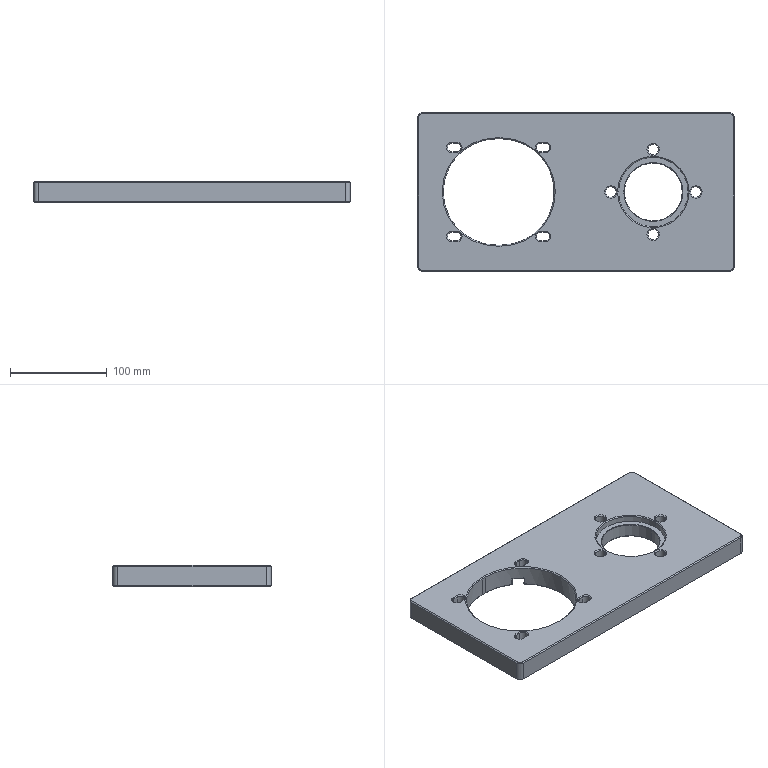NC program | NX | posted with a generic post | part box 328 x 164 x 22 mm
Lines 5345 to 6161 of 34171:
(ZLEVEL_PROFILE_1 , TOOL : D6)
N10634 T06 M6
N10636 G54
N10638 G17 G0 G90 X-32.492 Y47.462 S4500 M3
N10640 G43 Z30. H6
N10642 Z1.
N10644 G94 G1 X-36.544 Z0.788 F1600.
N10646 X-36.717 Y47.461 Z0.779
N10648 X-37.136 Y47.346 Z0.756
N10650 X-37.505 Y47.118 Z0.733
N10652 X-37.794 Y46.794 Z0.71
N10654 X-37.98 Y46.402 Z0.688
N10656 X-38.011 Y46.231 Z0.678
N10658 X-38.045 Y45.962 Z0.664
N10660 X-38.011 Y45.693 Z0.65
N10662 X-37.98 Y45.522 Z0.641
N10664 X-37.795 Y45.13 Z0.618
N10666 X-37.506 Y44.806 Z0.595
N10668 X-37.136 Y44.578 Z0.573
N10670 X-36.717 Y44.465 Z0.55
N10672 X-36.544 Y44.464 Z0.541
N10674 Y44.462
N10676 X-31.532 Z0.278
N10678 X-31.359 Y44.463 Z0.269
N10680 X-30.938 Y44.578 Z0.246
N10682 X-30.568 Y44.808 Z0.223
N10684 X-30.279 Y45.134 Z0.201
N10686 X-30.095 Y45.529 Z0.178
N10688 X-30.065 Y45.7 Z0.169
N10690 X-30.06 Y45.714 Z0.168
N10692 X-30.049 Y45.79 Z0.164
N10694 Y46.133 Z0.146
N10696 X-30.061 Y46.21 Z0.142
N10698 X-30.095 Y46.398 Z0.132
N10700 X-30.28 Y46.792 Z0.109
N10702 X-30.569 Y47.117 Z0.086
N10704 X-30.939 Y47.346 Z0.063
N10706 X-31.359 Y47.459 Z0.04
N10708 X-31.532 Y47.46 Z0.031
N10710 Y47.462
N10712 X-34.038 Z-0.1
N10714 X-36.544
N10716 G3 X-38.011 Y46.231 R1.504
N10718 G1 X-38.045 Y45.962
N10720 X-38.011 Y45.693
N10722 G3 X-36.544 Y44.464 R1.5
N10724 G1 Y44.462
N10726 X-31.532
N10728 G3 X-30.065 Y45.7 R1.5
N10730 G1 X-30.06 Y45.714
N10732 X-30.049 Y45.79
N10734 Y46.133
N10736 X-30.061 Y46.21
N10738 X-30.065 Y46.227
N10740 G3 X-31.532 Y47.46 R1.497
N10742 G1 Y47.462
N10744 X-34.038
N10746 X-36.397 Z-0.141
N10748 X-36.565 Y47.456 Z-0.144
N10750 X-36.733 Y47.446 Z-0.147
N10752 X-36.857 Y47.424 Z-0.149
N10754 X-36.918 Y47.412 Z-0.15
N10756 X-36.966 Y47.397 Z-0.151
N10758 X-37.06 Y47.367 Z-0.153
N10760 X-37.243 Y47.284 Z-0.156
N10762 X-37.36 Y47.215 Z-0.159
N10764 X-37.513 Y47.098 Z-0.162
N10766 X-37.618 Y46.999 Z-0.165
N10768 X-37.7 Y46.904 Z-0.167
N10770 X-37.739 Y46.855 Z-0.168
N10772 X-37.82 Y46.731 Z-0.171
N10774 X-37.884 Y46.61 Z-0.173
N10776 X-37.915 Y46.549 Z-0.174
N10778 X-37.931 Y46.508 Z-0.175
N10780 X-37.961 Y46.426 Z-0.176
N10782 X-37.998 Y46.297 Z-0.179
N10784 X-38.02 Y46.187 Z-0.181
N10786 X-38.029 Y46.096 Z-0.182
N10788 X-38.033 Y45.867 Z-0.186
N10790 X-38.024 Y45.761 Z-0.188
N10792 X-38.001 Y45.644 Z-0.19
N10794 X-37.988 Y45.586 Z-0.191
N10796 X-37.973 Y45.536 Z-0.192
N10798 X-37.938 Y45.436 Z-0.194
N10800 X-37.868 Y45.283 Z-0.197
N10802 X-37.787 Y45.136 Z-0.2
N10804 G3 X-36.544 Y44.464 R1.5
N10806 G1 Y44.462
N10808 X-31.532
N10810 G3 X-30.065 Y45.7 R1.5
N10812 G1 X-30.06 Y45.714
N10814 X-30.049 Y45.79
N10816 Y46.133
N10818 X-30.061 Y46.21
N10820 X-30.065 Y46.227
N10822 G3 X-31.532 Y47.46 R1.497
N10824 G1 Y47.462
N10826 X-34.038
N10828 X-36.397 Z-0.241
N10830 X-36.565 Y47.456 Z-0.244
N10832 X-36.733 Y47.446 Z-0.247
N10834 X-36.857 Y47.424 Z-0.249
N10836 X-36.918 Y47.412 Z-0.25
N10838 X-36.966 Y47.397 Z-0.251
N10840 X-37.06 Y47.367 Z-0.253
N10842 X-37.243 Y47.284 Z-0.256
N10844 X-37.36 Y47.215 Z-0.259
N10846 X-37.513 Y47.098 Z-0.262
N10848 X-37.618 Y46.999 Z-0.265
N10850 X-37.7 Y46.904 Z-0.267
N10852 X-37.739 Y46.855 Z-0.268
N10854 X-37.82 Y46.731 Z-0.271
N10856 X-37.884 Y46.61 Z-0.273
N10858 X-37.915 Y46.549 Z-0.274
N10860 X-37.931 Y46.508 Z-0.275
N10862 X-37.961 Y46.426 Z-0.276
N10864 X-37.998 Y46.297 Z-0.279
N10866 X-38.02 Y46.187 Z-0.281
N10868 X-38.029 Y46.096 Z-0.282
N10870 X-38.033 Y45.867 Z-0.286
N10872 X-38.024 Y45.761 Z-0.288
N10874 X-38.001 Y45.644 Z-0.29
N10876 X-37.988 Y45.586 Z-0.291
N10878 X-37.973 Y45.536 Z-0.292
N10880 X-37.938 Y45.436 Z-0.294
N10882 X-37.868 Y45.283 Z-0.297
N10884 X-37.787 Y45.136 Z-0.3
N10886 G3 X-36.544 Y44.464 R1.5
N10888 G1 Y44.462
N10890 X-31.532
N10892 G3 X-30.065 Y45.7 R1.5
N10894 G1 X-30.06 Y45.714
N10896 X-30.049 Y45.79
N10898 Y46.133
N10900 X-30.061 Y46.21
N10902 X-30.065 Y46.227
N10904 G3 X-31.532 Y47.46 R1.497
N10906 G1 Y47.462
N10908 X-34.038
N10910 X-36.397 Z-0.341
N10912 X-36.565 Y47.456 Z-0.344
N10914 X-36.733 Y47.446 Z-0.347
N10916 X-36.857 Y47.424 Z-0.349
N10918 X-36.918 Y47.412 Z-0.35
N10920 X-36.966 Y47.397 Z-0.351
N10922 X-37.06 Y47.367 Z-0.353
N10924 X-37.243 Y47.284 Z-0.356
N10926 X-37.36 Y47.215 Z-0.359
N10928 X-37.513 Y47.098 Z-0.362
N10930 X-37.618 Y46.999 Z-0.365
N10932 X-37.7 Y46.904 Z-0.367
N10934 X-37.739 Y46.855 Z-0.368
N10936 X-37.82 Y46.731 Z-0.371
N10938 X-37.884 Y46.61 Z-0.373
N10940 X-37.915 Y46.549 Z-0.374
N10942 X-37.931 Y46.508 Z-0.375
N10944 X-37.961 Y46.426 Z-0.376
N10946 X-37.998 Y46.297 Z-0.379
N10948 X-38.02 Y46.187 Z-0.381
N10950 X-38.029 Y46.096 Z-0.382
N10952 X-38.033 Y45.867 Z-0.386
N10954 X-38.024 Y45.761 Z-0.388
N10956 X-38.001 Y45.644 Z-0.39
N10958 X-37.988 Y45.586 Z-0.391
N10960 X-37.973 Y45.536 Z-0.392
N10962 X-37.938 Y45.436 Z-0.394
N10964 X-37.868 Y45.283 Z-0.397
N10966 X-37.787 Y45.136 Z-0.4
N10968 G3 X-36.544 Y44.464 R1.5
N10970 G1 Y44.462
N10972 X-31.532
N10974 G3 X-30.065 Y45.7 R1.5
N10976 G1 X-30.06 Y45.714
N10978 X-30.049 Y45.79
N10980 Y46.133
N10982 X-30.061 Y46.21
N10984 X-30.065 Y46.227
N10986 G3 X-31.532 Y47.46 R1.497
N10988 G1 Y47.462
N10990 X-34.038
N10992 X-36.397 Z-0.441
N10994 X-36.565 Y47.456 Z-0.444
N10996 X-36.733 Y47.446 Z-0.447
N10998 X-36.857 Y47.424 Z-0.449
N11000 X-36.918 Y47.412 Z-0.45
N11002 X-36.966 Y47.397 Z-0.451
N11004 X-37.06 Y47.367 Z-0.453
N11006 X-37.243 Y47.284 Z-0.456
N11008 X-37.36 Y47.215 Z-0.459
N11010 X-37.513 Y47.098 Z-0.462
N11012 X-37.618 Y46.999 Z-0.465
N11014 X-37.7 Y46.904 Z-0.467
N11016 X-37.739 Y46.855 Z-0.468
N11018 X-37.82 Y46.731 Z-0.471
N11020 X-37.884 Y46.61 Z-0.473
N11022 X-37.915 Y46.549 Z-0.474
N11024 X-37.931 Y46.508 Z-0.475
N11026 X-37.961 Y46.426 Z-0.476
N11028 X-37.998 Y46.297 Z-0.479
N11030 X-38.02 Y46.187 Z-0.481
N11032 X-38.029 Y46.096 Z-0.482
N11034 X-38.033 Y45.867 Z-0.486
N11036 X-38.024 Y45.761 Z-0.488
N11038 X-38.001 Y45.644 Z-0.49
N11040 X-37.988 Y45.586 Z-0.491
N11042 X-37.973 Y45.536 Z-0.492
N11044 X-37.938 Y45.436 Z-0.494
N11046 X-37.868 Y45.283 Z-0.497
N11048 X-37.787 Y45.136 Z-0.5
N11050 G3 X-36.544 Y44.464 R1.5
N11052 G1 Y44.462
N11054 X-31.532
N11056 G3 X-30.065 Y45.7 R1.5
N11058 G1 X-30.06 Y45.714
N11060 X-30.049 Y45.79
N11062 Y46.133
N11064 X-30.061 Y46.21
N11066 X-30.065 Y46.227
N11068 G3 X-31.532 Y47.46 R1.497
N11070 G1 Y47.462
N11072 X-34.038
N11074 X-36.397 Z-0.541
N11076 X-36.565 Y47.456 Z-0.544
N11078 X-36.733 Y47.446 Z-0.547
N11080 X-36.857 Y47.424 Z-0.549
N11082 X-36.918 Y47.412 Z-0.55
N11084 X-36.966 Y47.397 Z-0.551
N11086 X-37.06 Y47.367 Z-0.553
N11088 X-37.243 Y47.284 Z-0.556
N11090 X-37.36 Y47.215 Z-0.559
N11092 X-37.513 Y47.098 Z-0.562
N11094 X-37.618 Y46.999 Z-0.565
N11096 X-37.7 Y46.904 Z-0.567
N11098 X-37.739 Y46.855 Z-0.568
N11100 X-37.82 Y46.731 Z-0.571
N11102 X-37.884 Y46.61 Z-0.573
N11104 X-37.915 Y46.549 Z-0.574
N11106 X-37.931 Y46.508 Z-0.575
N11108 X-37.961 Y46.426 Z-0.576
N11110 X-37.998 Y46.297 Z-0.579
N11112 X-38.02 Y46.187 Z-0.581
N11114 X-38.029 Y46.096 Z-0.582
N11116 X-38.033 Y45.867 Z-0.586
N11118 X-38.024 Y45.761 Z-0.588
N11120 X-38.001 Y45.644 Z-0.59
N11122 X-37.988 Y45.586 Z-0.591
N11124 X-37.973 Y45.536 Z-0.592
N11126 X-37.938 Y45.436 Z-0.594
N11128 X-37.868 Y45.283 Z-0.597
N11130 X-37.787 Y45.136 Z-0.6
N11132 G3 X-36.544 Y44.464 R1.5
N11134 G1 Y44.462
N11136 X-31.532
N11138 G3 X-30.065 Y45.7 R1.5
N11140 G1 X-30.06 Y45.714
N11142 X-30.049 Y45.79
N11144 Y46.133
N11146 X-30.061 Y46.21
N11148 X-30.065 Y46.227
N11150 G3 X-31.532 Y47.46 R1.497
N11152 G1 Y47.462
N11154 X-34.038
N11156 X-36.397 Z-0.641
N11158 X-36.565 Y47.456 Z-0.644
N11160 X-36.733 Y47.446 Z-0.647
N11162 X-36.857 Y47.424 Z-0.649
N11164 X-36.918 Y47.412 Z-0.65
N11166 X-36.966 Y47.397 Z-0.651
N11168 X-37.06 Y47.367 Z-0.653
N11170 X-37.243 Y47.284 Z-0.656
N11172 X-37.36 Y47.215 Z-0.659
N11174 X-37.513 Y47.098 Z-0.662
N11176 X-37.618 Y46.999 Z-0.665
N11178 X-37.7 Y46.904 Z-0.667
N11180 X-37.739 Y46.855 Z-0.668
N11182 X-37.82 Y46.731 Z-0.671
N11184 X-37.884 Y46.61 Z-0.673
N11186 X-37.915 Y46.549 Z-0.674
N11188 X-37.931 Y46.508 Z-0.675
N11190 X-37.961 Y46.426 Z-0.676
N11192 X-37.998 Y46.297 Z-0.679
N11194 X-38.02 Y46.187 Z-0.681
N11196 X-38.029 Y46.096 Z-0.682
N11198 X-38.033 Y45.867 Z-0.686
N11200 X-38.024 Y45.761 Z-0.688
N11202 X-38.001 Y45.644 Z-0.69
N11204 X-37.988 Y45.586 Z-0.691
N11206 X-37.973 Y45.536 Z-0.692
N11208 X-37.938 Y45.436 Z-0.694
N11210 X-37.868 Y45.283 Z-0.697
N11212 X-37.787 Y45.136 Z-0.7
N11214 G3 X-36.544 Y44.464 R1.5
N11216 G1 Y44.462
N11218 X-31.532
N11220 G3 X-30.065 Y45.7 R1.5
N11222 G1 X-30.06 Y45.714
N11224 X-30.049 Y45.79
N11226 Y46.133
N11228 X-30.061 Y46.21
N11230 X-30.065 Y46.227
N11232 G3 X-31.532 Y47.46 R1.497
N11234 G1 Y47.462
N11236 X-34.038
N11238 X-36.397 Z-0.741
N11240 X-36.565 Y47.456 Z-0.744
N11242 X-36.733 Y47.446 Z-0.747
N11244 X-36.857 Y47.424 Z-0.749
N11246 X-36.918 Y47.412 Z-0.75
N11248 X-36.966 Y47.397 Z-0.751
N11250 X-37.06 Y47.367 Z-0.753
N11252 X-37.243 Y47.284 Z-0.756
N11254 X-37.36 Y47.215 Z-0.759
N11256 X-37.513 Y47.098 Z-0.762
N11258 X-37.618 Y46.999 Z-0.765
N11260 X-37.7 Y46.904 Z-0.767
N11262 X-37.739 Y46.855 Z-0.768
N11264 X-37.82 Y46.731 Z-0.771
N11266 X-37.884 Y46.61 Z-0.773
N11268 X-37.915 Y46.55 Z-0.774
N11270 X-37.93 Y46.509 Z-0.775
N11272 X-37.961 Y46.426 Z-0.776
N11274 X-38.011 Y46.227 Z-0.78
N11276 X-38.03 Y46.096 Z-0.782
N11278 X-38.035 Y45.894 Z-0.786
N11280 X-38.024 Y45.761 Z-0.788
N11282 X-38.001 Y45.644 Z-0.79
N11284 X-37.988 Y45.586 Z-0.791
N11286 X-37.973 Y45.535 Z-0.792
N11288 X-37.938 Y45.436 Z-0.794
N11290 X-37.868 Y45.283 Z-0.797
N11292 X-37.787 Y45.136 Z-0.8
N11294 G3 X-36.544 Y44.464 R1.5
N11296 G1 Y44.462
N11298 X-31.532
N11300 G3 X-30.065 Y45.7 R1.5
N11302 G1 X-30.06 Y45.714
N11304 X-30.049 Y45.79
N11306 Y46.133
N11308 X-30.061 Y46.21
N11310 X-30.065 Y46.227
N11312 G3 X-31.532 Y47.46 R1.497
N11314 G1 Y47.462
N11316 X-34.038
N11318 X-36.397 Z-0.841
N11320 X-36.565 Y47.456 Z-0.844
N11322 X-36.733 Y47.446 Z-0.847
N11324 X-36.857 Y47.424 Z-0.849
N11326 X-36.918 Y47.412 Z-0.85
N11328 X-36.966 Y47.397 Z-0.851
N11330 X-37.06 Y47.367 Z-0.853
N11332 X-37.243 Y47.284 Z-0.856
N11334 X-37.36 Y47.215 Z-0.859
N11336 X-37.513 Y47.098 Z-0.862
N11338 X-37.618 Y46.999 Z-0.865
N11340 X-37.7 Y46.904 Z-0.867
N11342 X-37.739 Y46.855 Z-0.868
N11344 X-37.82 Y46.731 Z-0.871
N11346 X-37.884 Y46.61 Z-0.873
N11348 X-37.915 Y46.55 Z-0.874
N11350 X-37.93 Y46.509 Z-0.875
N11352 X-37.961 Y46.426 Z-0.876
N11354 X-38.011 Y46.227 Z-0.88
N11356 X-38.03 Y46.096 Z-0.882
N11358 X-38.035 Y45.894 Z-0.886
N11360 X-38.024 Y45.761 Z-0.888
N11362 X-38.001 Y45.644 Z-0.89
N11364 X-37.988 Y45.586 Z-0.891
N11366 X-37.973 Y45.535 Z-0.892
N11368 X-37.938 Y45.436 Z-0.894
N11370 X-37.868 Y45.283 Z-0.897
N11372 X-37.787 Y45.136 Z-0.9
N11374 G3 X-36.544 Y44.464 R1.5
N11376 G1 Y44.462
N11378 X-31.532
N11380 G3 X-30.065 Y45.7 R1.5
N11382 G1 X-30.06 Y45.714
N11384 X-30.049 Y45.79
N11386 Y46.133
N11388 X-30.061 Y46.21
N11390 X-30.065 Y46.227
N11392 G3 X-31.532 Y47.46 R1.497
N11394 G1 Y47.462
N11396 X-34.038
N11398 X-36.397 Z-0.941
N11400 X-36.565 Y47.456 Z-0.944
N11402 X-36.733 Y47.447 Z-0.947
N11404 X-36.855 Y47.424 Z-0.949
N11406 X-36.915 Y47.412 Z-0.95
N11408 X-36.964 Y47.398 Z-0.951
N11410 X-37.06 Y47.367 Z-0.953
N11412 X-37.244 Y47.283 Z-0.956
N11414 X-37.36 Y47.215 Z-0.959
N11416 X-37.513 Y47.098 Z-0.962
N11418 X-37.618 Y46.999 Z-0.965
N11420 X-37.7 Y46.904 Z-0.967
N11422 X-37.739 Y46.855 Z-0.968
N11424 X-37.82 Y46.731 Z-0.971
N11426 X-37.884 Y46.61 Z-0.973
N11428 X-37.915 Y46.55 Z-0.974
N11430 X-37.931 Y46.509 Z-0.975
N11432 X-37.961 Y46.426 Z-0.976
N11434 X-37.998 Y46.295 Z-0.979
N11436 X-38.02 Y46.185 Z-0.981
N11438 X-38.029 Y46.096 Z-0.982
N11440 X-38.033 Y45.873 Z-0.986
N11442 X-38.023 Y45.762 Z-0.988
N11444 X-38. Y45.64 Z-0.99
N11446 X-37.987 Y45.579 Z-0.991
N11448 X-37.972 Y45.531 Z-0.992
N11450 X-37.938 Y45.436 Z-0.994
N11452 X-37.868 Y45.283 Z-0.997
N11454 X-37.789 Y45.135 Z-1.
N11456 G3 X-36.538 Y44.462 R1.5
N11458 G1 X-31.538
N11460 G3 X-30.038 Y45.962 R1.5
N11462 X-31.538 Y47.462 R1.5
N11464 G1 X-34.038
N11466 X-36.397 Z-1.041
N11468 X-36.565 Y47.456 Z-1.044
N11470 X-36.733 Y47.447 Z-1.047
N11472 X-36.916 Y47.413 Z-1.05
N11474 X-37.06 Y47.368 Z-1.053
N11476 X-37.18 Y47.315 Z-1.055
N11478 X-37.24 Y47.288 Z-1.056
N11480 X-37.28 Y47.265 Z-1.057
N11482 X-37.36 Y47.217 Z-1.059
N11484 X-37.523 Y47.089 Z-1.062
N11486 X-37.619 Y47.002 Z-1.065
N11488 X-37.729 Y46.869 Z-1.068
N11490 X-37.819 Y46.733 Z-1.071
N11492 X-37.91 Y46.558 Z-1.074
N11494 X-37.96 Y46.428 Z-1.076
N11496 X-38.01 Y46.233 Z-1.08
N11498 X-38.032 Y46.1 Z-1.082
N11500 X-38.037 Y45.908 Z-1.086
N11502 X-38.025 Y45.764 Z-1.088
N11504 X-38.002 Y45.648 Z-1.09
N11506 X-37.989 Y45.59 Z-1.091
N11508 X-37.975 Y45.539 Z-1.092
N11510 X-37.939 Y45.439 Z-1.094
N11512 X-37.869 Y45.286 Z-1.097
N11514 X-37.791 Y45.138 Z-1.1
N11516 G3 X-36.538 Y44.462 R1.5
N11518 G1 X-31.538
N11520 G3 X-30.038 Y45.962 R1.5
N11522 X-31.538 Y47.462 R1.5
N11524 G1 X-34.038
N11526 X-36.397 Z-1.141
N11528 X-36.565 Y47.456 Z-1.144
N11530 X-36.733 Y47.447 Z-1.147
N11532 X-36.916 Y47.413 Z-1.15
N11534 X-37.06 Y47.368 Z-1.153
N11536 X-37.18 Y47.315 Z-1.155
N11538 X-37.24 Y47.288 Z-1.156
N11540 X-37.28 Y47.265 Z-1.157
N11542 X-37.36 Y47.217 Z-1.159
N11544 X-37.523 Y47.089 Z-1.162
N11546 X-37.619 Y47.002 Z-1.165
N11548 X-37.729 Y46.869 Z-1.168
N11550 X-37.819 Y46.733 Z-1.171
N11552 X-37.91 Y46.558 Z-1.174
N11554 X-37.96 Y46.428 Z-1.176
N11556 X-38.01 Y46.233 Z-1.18
N11558 X-38.032 Y46.1 Z-1.182
N11560 X-38.037 Y45.908 Z-1.186
N11562 X-38.025 Y45.764 Z-1.188
N11564 X-38.002 Y45.648 Z-1.19
N11566 X-37.989 Y45.59 Z-1.191
N11568 X-37.975 Y45.539 Z-1.192
N11570 X-37.939 Y45.439 Z-1.194
N11572 X-37.869 Y45.286 Z-1.197
N11574 X-37.791 Y45.138 Z-1.2
N11576 G3 X-36.538 Y44.462 R1.5
N11578 G1 X-31.538
N11580 G3 X-30.038 Y45.962 R1.5
N11582 X-31.538 Y47.462 R1.5
N11584 G1 X-34.038
N11586 X-36.397 Z-1.241
N11588 X-36.565 Y47.456 Z-1.244
N11590 X-36.733 Y47.447 Z-1.247
N11592 X-36.916 Y47.413 Z-1.25
N11594 X-37.06 Y47.368 Z-1.253
N11596 X-37.18 Y47.315 Z-1.255
N11598 X-37.24 Y47.288 Z-1.256
N11600 X-37.28 Y47.265 Z-1.257
N11602 X-37.36 Y47.217 Z-1.259
N11604 X-37.523 Y47.089 Z-1.262
N11606 X-37.619 Y47.002 Z-1.265
N11608 X-37.729 Y46.869 Z-1.268
N11610 X-37.819 Y46.733 Z-1.271
N11612 X-37.91 Y46.558 Z-1.274
N11614 X-37.96 Y46.428 Z-1.276
N11616 X-38.01 Y46.233 Z-1.28
N11618 X-38.032 Y46.1 Z-1.282
N11620 X-38.037 Y45.908 Z-1.286
N11622 X-38.025 Y45.764 Z-1.288
N11624 X-38.002 Y45.648 Z-1.29
N11626 X-37.989 Y45.59 Z-1.291
N11628 X-37.975 Y45.539 Z-1.292
N11630 X-37.939 Y45.439 Z-1.294
N11632 X-37.869 Y45.286 Z-1.297
N11634 X-37.791 Y45.138 Z-1.3
N11636 G3 X-36.538 Y44.462 R1.5
N11638 G1 X-31.538
N11640 G3 X-30.038 Y45.962 R1.5
N11642 X-31.538 Y47.462 R1.5
N11644 G1 X-34.038
N11646 X-36.397 Z-1.341
N11648 X-36.565 Y47.456 Z-1.344
N11650 X-36.733 Y47.447 Z-1.347
N11652 X-36.916 Y47.413 Z-1.35
N11654 X-37.06 Y47.368 Z-1.353
N11656 X-37.18 Y47.315 Z-1.355
N11658 X-37.24 Y47.288 Z-1.356
N11660 X-37.28 Y47.265 Z-1.357
N11662 X-37.36 Y47.217 Z-1.359
N11664 X-37.523 Y47.089 Z-1.362
N11666 X-37.619 Y47.002 Z-1.365
N11668 X-37.729 Y46.869 Z-1.368
N11670 X-37.819 Y46.733 Z-1.371
N11672 X-37.91 Y46.558 Z-1.374
N11674 X-37.96 Y46.428 Z-1.376
N11676 X-38.01 Y46.233 Z-1.38
N11678 X-38.032 Y46.1 Z-1.382
N11680 X-38.037 Y45.908 Z-1.386
N11682 X-38.025 Y45.764 Z-1.388
N11684 X-38.002 Y45.648 Z-1.39
N11686 X-37.989 Y45.59 Z-1.391
N11688 X-37.975 Y45.539 Z-1.392
N11690 X-37.939 Y45.439 Z-1.394
N11692 X-37.869 Y45.286 Z-1.397
N11694 X-37.791 Y45.138 Z-1.4
N11696 G3 X-36.538 Y44.462 R1.5
N11698 G1 X-31.538
N11700 G3 X-30.038 Y45.962 R1.5
N11702 X-31.538 Y47.462 R1.5
N11704 G1 X-34.038
N11706 X-36.397 Z-1.441
N11708 X-36.565 Y47.456 Z-1.444
N11710 X-36.733 Y47.447 Z-1.447
N11712 X-36.916 Y47.413 Z-1.45
N11714 X-37.06 Y47.368 Z-1.453
N11716 X-37.18 Y47.315 Z-1.455
N11718 X-37.24 Y47.288 Z-1.456
N11720 X-37.28 Y47.265 Z-1.457
N11722 X-37.36 Y47.217 Z-1.459
N11724 X-37.523 Y47.089 Z-1.462
N11726 X-37.619 Y47.002 Z-1.465
N11728 X-37.728 Y46.869 Z-1.468
N11730 X-37.819 Y46.733 Z-1.471
N11732 X-37.91 Y46.558 Z-1.474
N11734 X-37.96 Y46.428 Z-1.476
N11736 X-38.01 Y46.233 Z-1.48
N11738 X-38.032 Y46.1 Z-1.482
N11740 X-38.037 Y45.908 Z-1.486
N11742 X-38.025 Y45.764 Z-1.488
N11744 X-38.002 Y45.648 Z-1.49
N11746 X-37.989 Y45.59 Z-1.491
N11748 X-37.975 Y45.539 Z-1.492
N11750 X-37.939 Y45.439 Z-1.494
N11752 X-37.869 Y45.286 Z-1.497
N11754 X-37.791 Y45.138 Z-1.5
N11756 G3 X-36.538 Y44.462 R1.5
N11758 G1 X-31.538
N11760 G3 X-30.038 Y45.962 R1.5
N11762 X-31.538 Y47.462 R1.5
N11764 G1 X-34.038
N11766 X-36.397 Z-1.541
N11768 X-36.565 Y47.456 Z-1.544
N11770 X-36.733 Y47.447 Z-1.547
N11772 X-36.916 Y47.413 Z-1.55
N11774 X-37.06 Y47.368 Z-1.553
N11776 X-37.18 Y47.315 Z-1.555
N11778 X-37.24 Y47.288 Z-1.556
N11780 X-37.28 Y47.265 Z-1.557
N11782 X-37.36 Y47.217 Z-1.559
N11784 X-37.523 Y47.089 Z-1.562
N11786 X-37.619 Y47.002 Z-1.565
N11788 X-37.728 Y46.869 Z-1.568
N11790 X-37.819 Y46.733 Z-1.571
N11792 X-37.91 Y46.558 Z-1.574
N11794 X-37.96 Y46.428 Z-1.576
N11796 X-38.01 Y46.233 Z-1.58
N11798 X-38.032 Y46.1 Z-1.582
N11800 X-38.037 Y45.908 Z-1.586
N11802 X-38.025 Y45.764 Z-1.588
N11804 X-38.002 Y45.648 Z-1.59
N11806 X-37.989 Y45.59 Z-1.591
N11808 X-37.975 Y45.539 Z-1.592
N11810 X-37.939 Y45.439 Z-1.594
N11812 X-37.869 Y45.286 Z-1.597
N11814 X-37.791 Y45.138 Z-1.6
N11816 G3 X-36.538 Y44.462 R1.5
N11818 G1 X-31.538
N11820 G3 X-30.038 Y45.962 R1.5
N11822 X-31.538 Y47.462 R1.5
N11824 G1 X-34.038
N11826 X-36.397 Z-1.641
N11828 X-36.565 Y47.456 Z-1.644
N11830 X-36.733 Y47.447 Z-1.647
N11832 X-36.916 Y47.413 Z-1.65
N11834 X-37.06 Y47.368 Z-1.653
N11836 X-37.18 Y47.315 Z-1.655
N11838 X-37.24 Y47.288 Z-1.656
N11840 X-37.28 Y47.265 Z-1.657
N11842 X-37.36 Y47.217 Z-1.659
N11844 X-37.523 Y47.089 Z-1.662
N11846 X-37.619 Y47.002 Z-1.665
N11848 X-37.728 Y46.869 Z-1.668
N11850 X-37.819 Y46.733 Z-1.671
N11852 X-37.91 Y46.558 Z-1.674
N11854 X-37.96 Y46.428 Z-1.676
N11856 X-38.01 Y46.233 Z-1.68
N11858 X-38.032 Y46.1 Z-1.682
N11860 X-38.037 Y45.908 Z-1.686
N11862 X-38.025 Y45.764 Z-1.688
N11864 X-38.002 Y45.648 Z-1.69
N11866 X-37.989 Y45.59 Z-1.691
N11868 X-37.975 Y45.539 Z-1.692
N11870 X-37.939 Y45.439 Z-1.694
N11872 X-37.869 Y45.286 Z-1.697
N11874 X-37.791 Y45.138 Z-1.7
N11876 G3 X-36.538 Y44.462 R1.5
N11878 G1 X-31.538
N11880 G3 X-30.038 Y45.962 R1.5
N11882 X-31.538 Y47.462 R1.5
N11884 G1 X-34.038
N11886 X-36.397 Z-1.741
N11888 X-36.565 Y47.456 Z-1.744
N11890 X-36.733 Y47.447 Z-1.747
N11892 X-36.916 Y47.413 Z-1.75
N11894 X-37.06 Y47.368 Z-1.753
N11896 X-37.18 Y47.315 Z-1.755
N11898 X-37.24 Y47.288 Z-1.756
N11900 X-37.28 Y47.265 Z-1.757
N11902 X-37.36 Y47.217 Z-1.759
N11904 X-37.523 Y47.089 Z-1.762
N11906 X-37.619 Y47.002 Z-1.765
N11908 X-37.728 Y46.869 Z-1.768
N11910 X-37.819 Y46.733 Z-1.771
N11912 X-37.91 Y46.558 Z-1.774
N11914 X-37.96 Y46.428 Z-1.776
N11916 X-38.01 Y46.233 Z-1.78
N11918 X-38.032 Y46.1 Z-1.782
N11920 X-38.037 Y45.908 Z-1.786
N11922 X-38.025 Y45.764 Z-1.788
N11924 X-38.002 Y45.648 Z-1.79
N11926 X-37.989 Y45.59 Z-1.791
N11928 X-37.975 Y45.539 Z-1.792
N11930 X-37.939 Y45.439 Z-1.794
N11932 X-37.869 Y45.286 Z-1.797
N11934 X-37.791 Y45.138 Z-1.8
N11936 G3 X-36.538 Y44.462 R1.5
N11938 G1 X-31.538
N11940 G3 X-30.038 Y45.962 R1.5
N11942 X-31.538 Y47.462 R1.5
N11944 G1 X-34.038
N11946 X-36.397 Z-1.841
N11948 X-36.565 Y47.456 Z-1.844
N11950 X-36.733 Y47.447 Z-1.847
N11952 X-36.916 Y47.413 Z-1.85
N11954 X-37.06 Y47.368 Z-1.853
N11956 X-37.18 Y47.315 Z-1.855
N11958 X-37.24 Y47.288 Z-1.856
N11960 X-37.28 Y47.265 Z-1.857
N11962 X-37.36 Y47.217 Z-1.859
N11964 X-37.523 Y47.089 Z-1.862
N11966 X-37.619 Y47.002 Z-1.865
N11968 X-37.728 Y46.869 Z-1.868
N11970 X-37.819 Y46.733 Z-1.871
N11972 X-37.91 Y46.558 Z-1.874
N11974 X-37.96 Y46.428 Z-1.876
N11976 X-38.01 Y46.233 Z-1.88
N11978 X-38.032 Y46.1 Z-1.882
N11980 X-38.037 Y45.908 Z-1.886
N11982 X-38.025 Y45.764 Z-1.888
N11984 X-38.002 Y45.648 Z-1.89
N11986 X-37.989 Y45.59 Z-1.891
N11988 X-37.975 Y45.539 Z-1.892
N11990 X-37.939 Y45.439 Z-1.894
N11992 X-37.869 Y45.286 Z-1.897
N11994 X-37.791 Y45.138 Z-1.9
N11996 G3 X-36.538 Y44.462 R1.5
N11998 G1 X-31.538
N12000 G3 X-30.038 Y45.962 R1.5
N12002 X-31.538 Y47.462 R1.5
N12004 G1 X-34.038
N12006 X-36.397 Z-1.941
N12008 X-36.565 Y47.456 Z-1.944
N12010 X-36.733 Y47.447 Z-1.947
N12012 X-36.916 Y47.413 Z-1.95
N12014 X-37.06 Y47.368 Z-1.953
N12016 X-37.18 Y47.315 Z-1.955
N12018 X-37.24 Y47.288 Z-1.956
N12020 X-37.28 Y47.265 Z-1.957
N12022 X-37.36 Y47.217 Z-1.959
N12024 X-37.522 Y47.089 Z-1.962
N12026 X-37.619 Y47.002 Z-1.965
N12028 X-37.728 Y46.869 Z-1.968
N12030 X-37.819 Y46.733 Z-1.971
N12032 X-37.91 Y46.558 Z-1.974
N12034 X-37.96 Y46.428 Z-1.976
N12036 X-38.01 Y46.233 Z-1.98
N12038 X-38.032 Y46.1 Z-1.982
N12040 X-38.037 Y45.908 Z-1.986
N12042 X-38.025 Y45.764 Z-1.988
N12044 X-38.002 Y45.648 Z-1.99
N12046 X-37.989 Y45.59 Z-1.991
N12048 X-37.975 Y45.539 Z-1.992
N12050 X-37.939 Y45.439 Z-1.994
N12052 X-37.869 Y45.286 Z-1.997
N12054 X-37.791 Y45.138 Z-2.
N12056 G3 X-36.538 Y44.462 R1.5
N12058 G1 X-31.538
N12060 G3 X-30.038 Y45.962 R1.5
N12062 X-31.538 Y47.462 R1.5
N12064 G1 X-34.038
N12066 X-36.397 Z-2.041
N12068 X-36.565 Y47.456 Z-2.044
N12070 X-36.733 Y47.447 Z-2.047
N12072 X-36.916 Y47.413 Z-2.05
N12074 X-37.06 Y47.368 Z-2.053
N12076 X-37.18 Y47.315 Z-2.055
N12078 X-37.24 Y47.288 Z-2.056
N12080 X-37.28 Y47.265 Z-2.057
N12082 X-37.36 Y47.217 Z-2.059
N12084 X-37.522 Y47.089 Z-2.062
N12086 X-37.619 Y47.002 Z-2.065
N12088 X-37.728 Y46.869 Z-2.068
N12090 X-37.819 Y46.733 Z-2.071
N12092 X-37.91 Y46.558 Z-2.074
N12094 X-37.96 Y46.428 Z-2.076
N12096 X-38.01 Y46.233 Z-2.08
N12098 X-38.032 Y46.1 Z-2.082
N12100 X-38.037 Y45.908 Z-2.086
N12102 X-38.025 Y45.764 Z-2.088
N12104 X-38.002 Y45.648 Z-2.09
N12106 X-37.989 Y45.59 Z-2.091
N12108 X-37.975 Y45.539 Z-2.092
N12110 X-37.939 Y45.439 Z-2.094
N12112 X-37.869 Y45.286 Z-2.097
N12114 X-37.791 Y45.138 Z-2.1
N12116 G3 X-36.538 Y44.462 R1.5
N12118 G1 X-31.538
N12120 G3 X-30.038 Y45.962 R1.5
N12122 X-31.538 Y47.462 R1.5
N12124 G1 X-34.038
N12126 X-36.397 Z-2.141
N12128 X-36.565 Y47.456 Z-2.144
N12130 X-36.733 Y47.447 Z-2.147
N12132 X-36.916 Y47.413 Z-2.15
N12134 X-37.06 Y47.368 Z-2.153
N12136 X-37.18 Y47.315 Z-2.155
N12138 X-37.24 Y47.288 Z-2.156
N12140 X-37.28 Y47.265 Z-2.157
N12142 X-37.36 Y47.217 Z-2.159
N12144 X-37.522 Y47.089 Z-2.162
N12146 X-37.619 Y47.002 Z-2.165
N12148 X-37.728 Y46.869 Z-2.168
N12150 X-37.819 Y46.733 Z-2.171
N12152 X-37.91 Y46.558 Z-2.174
N12154 X-37.96 Y46.428 Z-2.176
N12156 X-38.01 Y46.233 Z-2.18
N12158 X-38.032 Y46.1 Z-2.182
N12160 X-38.037 Y45.908 Z-2.186
N12162 X-38.025 Y45.764 Z-2.188
N12164 X-38.002 Y45.648 Z-2.19
N12166 X-37.989 Y45.59 Z-2.191
N12168 X-37.975 Y45.539 Z-2.192
N12170 X-37.939 Y45.439 Z-2.194
N12172 X-37.869 Y45.286 Z-2.197
N12174 X-37.791 Y45.138 Z-2.2
N12176 G3 X-36.538 Y44.462 R1.5
N12178 G1 X-31.538
N12180 G3 X-30.038 Y45.962 R1.5
N12182 X-31.538 Y47.462 R1.5
N12184 G1 X-34.038
N12186 X-36.397 Z-2.241
N12188 X-36.565 Y47.456 Z-2.244
N12190 X-36.733 Y47.447 Z-2.247
N12192 X-36.916 Y47.413 Z-2.25
N12194 X-37.06 Y47.368 Z-2.253
N12196 X-37.18 Y47.315 Z-2.255
N12198 X-37.24 Y47.288 Z-2.256
N12200 X-37.28 Y47.265 Z-2.257
N12202 X-37.36 Y47.217 Z-2.259
N12204 X-37.522 Y47.089 Z-2.262
N12206 X-37.619 Y47.002 Z-2.265
N12208 X-37.728 Y46.869 Z-2.268
N12210 X-37.819 Y46.733 Z-2.271
N12212 X-37.91 Y46.558 Z-2.274
N12214 X-37.96 Y46.428 Z-2.276
N12216 X-38.01 Y46.233 Z-2.28
N12218 X-38.032 Y46.1 Z-2.282
N12220 X-38.037 Y45.908 Z-2.286
N12222 X-38.025 Y45.764 Z-2.288
N12224 X-38.002 Y45.648 Z-2.29
N12226 X-37.989 Y45.59 Z-2.291
N12228 X-37.975 Y45.539 Z-2.292
N12230 X-37.939 Y45.439 Z-2.294
N12232 X-37.869 Y45.286 Z-2.297
N12234 X-37.791 Y45.138 Z-2.3
N12236 G3 X-36.538 Y44.462 R1.5
N12238 G1 X-31.538
N12240 G3 X-30.038 Y45.962 R1.5
N12242 X-31.538 Y47.462 R1.5
N12244 G1 X-34.038
N12246 X-36.397 Z-2.341
N12248 X-36.565 Y47.456 Z-2.344
N12250 X-36.733 Y47.447 Z-2.347
N12252 X-36.916 Y47.413 Z-2.35
N12254 X-37.06 Y47.368 Z-2.353
N12256 X-37.18 Y47.315 Z-2.355
N12258 X-37.24 Y47.288 Z-2.356
N12260 X-37.28 Y47.265 Z-2.357